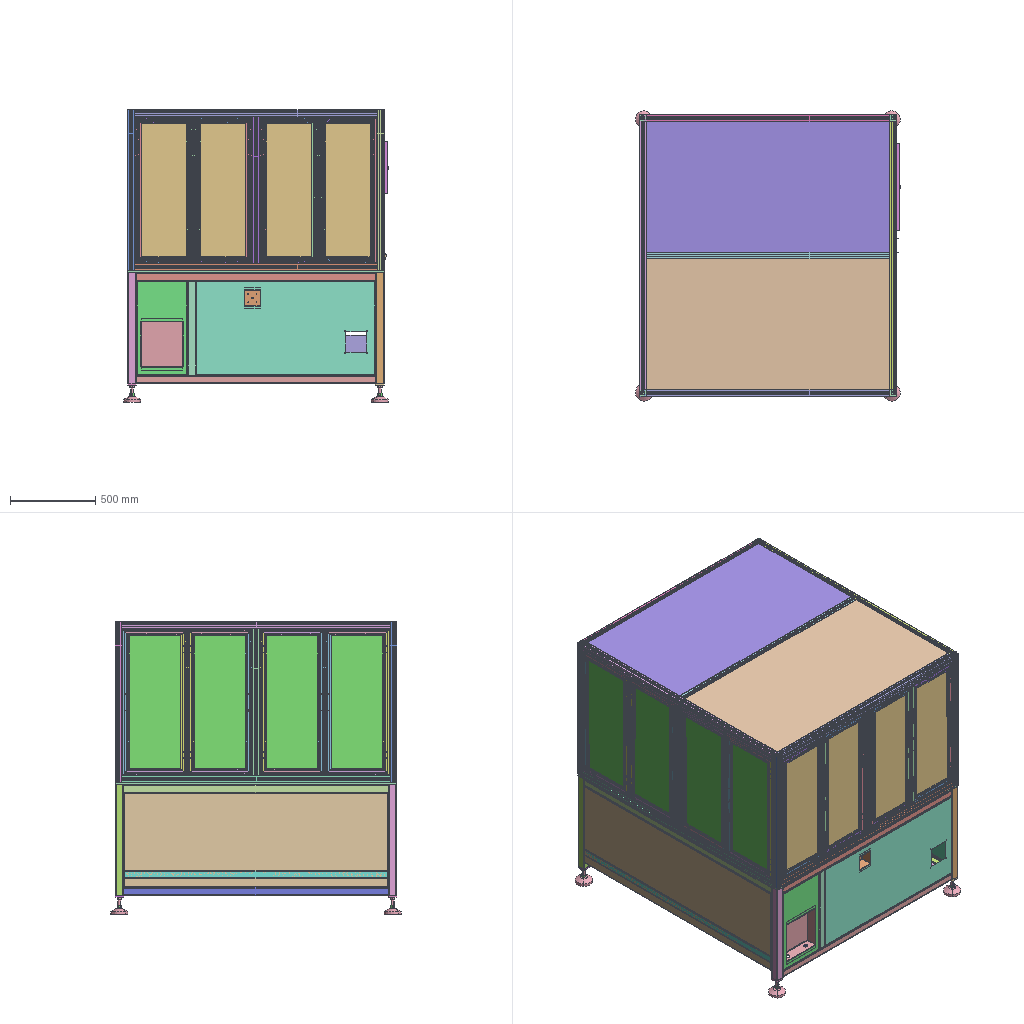Assembly | SolidWorks | 238 different items | 623 placed | box 1551 x 1700 x 1714 mm
Parts list (item | name | quantity | parent item | size | volume | features):
1 | (subassembly) | x2 | in 5 | 67.5 x 39 x 23.5 mm | 30109 mm3 | -
2 | (subassembly) | x1 | in 11 | 129 x 76.75 x 37 mm | 182069 mm3 | -
3 | (subassembly) | x2 | in 5, 21 | 99 x 76.75 x 37 mm | 182069 mm3 | -
4 | (subassembly) | x1 | in 21 | 152.5 x 57 x 74 mm | 389553 mm3 | -
5 | (subassembly) | x1 | - | 250 x 596.5 x 482 mm | 2400712 mm3 | -
6 | (subassembly) | x1 | in 15 | 103.415 x 32 x 20.8 mm | 30236 mm3 | -
7 | (subassembly) | x1 | in 15 | 10 x 102.865 x 20 mm | 11482 mm3 | -
8 | (subassembly) | x1 | in 36 | 226 x 45 x 54 mm | 65576 mm3 | -
9 | (subassembly) | x1 | in 37 | 181 x 45 x 54 mm | 67508 mm3 | -
10 | (subassembly) | x1 | in 37 | 83 x 83 x 36 mm | 177005 mm3 | -
11 | (subassembly) | x1 | - | - | 7253169 mm3 | -
12 | (subassembly) | x2 | in 35 | 83 x 83 x 36 mm | 177005 mm3 | features AEMSimFeature 1
13 | (subassembly) | x1 | - | - | 1570988 mm3 | features 3DProfileFeature 1
14 | (subassembly) | x1 | in 13 | 65 x 253 x 120 mm | 447705 mm3 | -
15 | (subassembly) | x1 | in 16 | 159.5 x 226.8 x 118.648 mm | 777455 mm3 | -
16 | (subassembly) | x1 | - | 159.5 x 226.8 x 118.648 mm | 777455 mm3 | -
17 | (subassembly) | x2 | in 18 | 102.5 x 118.189 x 195.029 mm | 527547 mm3 | -
18 | (subassembly) | x2 | - | 263 x 234.482 x 189.769 mm | 1000691 mm3 | -
19 | (subassembly) | x1 | - | - | - | features ReferencePattern 15, LocalCirPattern 2
20 | (subassembly) | x6 | in 19 | 80 x 60 x 32.8 mm | 73982 mm3 | features InContextFeatHolder 6
21 | (subassembly) | x1 | - | 353.5 x 596.5 x 482 mm | 3186701 mm3 | -
22 | (subassembly) | x1 | in 32 | 157 x 64 x 71 mm | 285801 mm3 | -
23 | (subassembly) | x1 | - | - | 100211807 mm3 | features ReferencePattern 10, MirrorCompFeat 4
24 | (subassembly) | x6 | in 19 | 40 x 111 x 58 mm | 78874 mm3 | features AEMSimFeature 1
25 | (subassembly) | x2 | - | 416.776 x 240 x 301.448 mm | 7009684 mm3 | -
26 | (subassembly) | x1 | - | 446.235 x 240 x 306.436 mm | 7009684 mm3 | -
27 | (subassembly) | x2 | in 5, 21 | 226 x 45 x 54 mm | 65576 mm3 | -
28 | (subassembly) | x1 | in 26 | 250 x 240 x 250 mm | 5886519 mm3 | -
29 | (subassembly) | x2 | in 25 | 250 x 240 x 250 mm | 5886519 mm3 | -
30 | (subassembly) | x6 | in 20 | 36 x 34.75 x 6.9 mm | 2892 mm3 | -
31 | (subassembly) | x1 | in 36 | 99 x 76.75 x 37 mm | 182069 mm3 | -
32 | (subassembly) | x1 | - | 285 x 559 x 312.685 mm | 2790889 mm3 | features ReferencePattern 5, CompositeCurve 2, MirrorCompFeat 1
33 | (subassembly) | x1 | in 36 | 152.5 x 57 x 74 mm | 389553 mm3 | -
34 | (subassembly) | x1 | - | 121 x 182 x 331.393 mm | 727155 mm3 | -
35 | (subassembly) | x2 | - | 121 x 83 x 36 mm | 201271 mm3 | -
36 | (subassembly) | x1 | - | 353.5 x 596.5 x 482 mm | 3186701 mm3 | features 3DProfileFeature 1
37 | (subassembly) | x1 | in 34 | 121 x 182 x 331.393 mm | 727155 mm3 | -
38 | - | x1 | in 22 | 157 x 50 x 50 mm | 85100 mm3 | features BaseBody 1
39 | - | x1 | - | 450 x 85 x 12 mm | 456645 mm3 | features BaseBody 1
40 | - | x1 | in 11 | 318 x 12 x 90 mm | 338579 mm3 | features HoleWzd 4, Chamfer 1, Extrusion 1
41 | - | x1 | - | 318 x 12 x 90 mm | 338579 mm3 | features BaseBody 1
42 | - | x1 | in 11 | 130 x 12 x 170 mm | 194409 mm3 | features HoleWzd 5, Chamfer 1, Extrusion 1
43 | - | x1 | - | 130 x 12 x 170 mm | 194409 mm3 | features BaseBody 1
44 | - | x1 | in 11 | 12 x 121.5 x 76 mm | 106329 mm3 | features HoleWzd 4, Chamfer 1, Extrusion 1
45 | - | x1 | - | 12 x 121.5 x 76 mm | 106329 mm3 | features BaseBody 1
46 | - | x1 | in 11 | 70 x 90 x 12 mm | 50116 mm3 | features HoleWzd 2, Chamfer 1, Extrusion 1
47 | - | x1 | - | 70 x 90 x 12 mm | 50116 mm3 | features BaseBody 1
48 | - | x1 | in 11 | 67 x 12 x 65 mm | 49086 mm3 | features HoleWzd 3, Extrusion 1
49 | - | x1 | in 22 | 80.5 x 71 x 64 mm | 175282 mm3 | features BaseBody 1
50 | - | x1 | - | 67 x 12 x 65 mm | 49086 mm3 | features BaseBody 1
51 | - | x2 | in 36 | 34 x 23.7 x 66.7 mm | 38485 mm3 | features BaseBody 2
52 | - | x2 | in 36 | 15 x 15 x 280 mm | 57550 mm3 | features BaseBody 1
53 | - | x1 | in 13 | - | - | features BaseBody 3, RefSurface 1
54 | - | x1 | in 13 | - | - | features BaseBody 14, RefSurface 4
55 | - | x1 | in 13 | 292.891 x 46.5 x 70 mm | 38586 mm3 | features BaseBody 7
56 | - | x1 | in 36 | 15 x 15 x 25 mm | 4329 mm3 | features BaseBody 1
57 | - | x4 | in 17 | 15 x 2.5 x 45 mm | 1095 mm3 | features BaseBody 1
58 | - | x2 | in 17 | 160 x 30 x 56 mm | 169757 mm3 | features BaseBody 1
59 | - | x4 | in 17 | 153.66 x 6 x 80 mm | 57575 mm3 | features BaseBody 1
60 | - | x2 | in 37 | 34 x 23.7 x 66.7 mm | 38485 mm3 | features BaseBody 2
61 | - | x12 | in 17 | 46 x 2 x 10 mm | 787.268 mm3 | features BaseBody 1
62 | - | x32 | in 17 | 46 x 0.5 x 10 mm | 196.817 mm3 | features BaseBody 1
63 | - | x2 | in 17 | 80 x 15 x 180 mm | 182488 mm3 | features BaseBody 1
64 | - | x4 | in 17 | 46 x 2 x 70 mm | 6168 mm3 | features BaseBody 1
65 | - | x4 | in 17 | 46 x 1.5 x 102 mm | 6734 mm3 | features BaseBody 1
66 | - | x2 | in 37 | 15 x 15 x 280 mm | 57550 mm3 | features BaseBody 1
67 | - | x2 | in 18 | 116 x 15 x 60 mm | 18438 mm3 | features BaseBody 1
68 | - | x2 | in 18 | 189.769 x 2 x 46.25 mm | 14558 mm3 | features BaseBody 1
69 | - | x2 | in 18 | 263 x 106.293 x 188.106 mm | 187834 mm3 | features BaseBody 1
70 | - | x2 | in 32 | 12 x 12 x 40 mm | 4457 mm3 | features Extrusion 1, RevCut 1
71 | - | x1 | in 36 | 28 x 30 x 10 mm | 7787 mm3 | features BaseBody 1
72 | - | x1 | in 19 | 700 x 690 x 12 mm | 4521944 mm3 | features CirPattern 5, ICE 3, HoleWzd 2, Extrusion 1
73 | - | x1 | in 23 | 1500 x 1650 x 672 mm | 49489000 mm3 | features ICE 14, FlatPattern 12, EdgeFlange 11, HoleWzd 11, SMBaseFlange 9, SheetMetal 9, MirrorSolid 6, MirrorPattern 4, Fillet 3, MoveCopyBody 2, MoveFace 2, WeldCornerFeat 2, 3DProfileFeature 1, Chamfer 1, EndCap 1, WeldMemberFeat 1, WeldmentFeature 1
74 | - | x6 | in 20 | 60 x 50 x 32 mm | 31490 mm3 | features Cut 4, ICE 4, Extrusion 1, Fillet 1, MirrorPattern 1
75 | - | x6 | in 20 | 80 x 60 x 20 mm | 39600 mm3 | features ICE 2, Extrusion 1
76 | - | x2 | - | 250 x 134 x 174.039 mm | 134233 mm3 | features BaseBody 3
77 | - | x1 | in 23 | 1500 x 1650 x 942 mm | 12502911 mm3 | features WeldCornerFeat 2, 3DProfileFeature 1, ICE 1, MirrorSolid 1, WeldMemberFeat 1, WeldmentFeature 1
78 | - | x5 | in 23 | 379.5 x 856 x 20 mm | 2107206 mm3 | features HoleWzd 3, ICE 1, WeldMemberFeat 1, WeldmentFeature 1
79 | - | x2 | in 35 | 80 x 30 x 10 mm | 23980 mm3 | features Extrusion 1, ICE 1
80 | - | x4 | in 35 | 2.5 x 2.5 x 30 mm | 142.655 mm3 | features Chamfer 1, Extrusion 1
81 | - | x1 | in 23 | 379.5 x 856 x 20 mm | 2241124 mm3 | features HoleWzd 3, ICE 3, WeldMemberFeat 1, WeldmentFeature 1
82 | - | x1 | - | 20 x 20 x 65 mm | 20420 mm3 | features BaseBody 1
83 | - | x8 | in 23 | 341.5 x 856 x 20 mm | 1950280 mm3 | features HoleWzd 3, ICE 1, WeldMemberFeat 1, WeldmentFeature 1
84 | - | x1 | in 23 | 764 x 860 x 5 mm | 2935200 mm3 | features Extrusion 1, ICE 1
85 | - | x2 | in 23 | 384.5 x 547 x 21.5 mm | 378210 mm3 | features EdgeFlange 3, ICE 2, Fillet 1, FlatPattern 1, SMBaseFlange 1, SheetMetal 1
86 | - | x2 | in 23 | 371 x 547 x 20 mm | 376908 mm3 | features EdgeFlange 2, ICE 2, FlatPattern 1, SMBaseFlange 1, SheetMetal 1
87 | - | x1 | in 37 | 180 x 30 x 20 mm | 107950 mm3 | features Extrusion 1, ICE 1
88 | - | x2 | in 37 | 4 x 4 x 20 mm | 251.327 mm3 | features Extrusion 1
89 | - | x6 | in 19 | 25 x 40 x 18 mm | 6202 mm3 | features ICE 2, Chamfer 1, Extrusion 1
90 | - | x6 | in 5, 21, 36 | 60 x 34 x 15 mm | 30600 mm3 | features Extrusion 1
91 | - | x1 | in 21 | 28 x 30 x 10 mm | 7787 mm3 | features BaseBody 1
92 | - | x1 | in 37 | 180 x 100 x 10 mm | 124316 mm3 | features Extrusion 1, HoleWzd 1, ICE 1
93 | - | x4 | in 12 | 40.5 x 5.8 x 4.4 mm | 628.814 mm3 | features BaseBody 1
94 | - | x1 | in 37 | 23 x 30 x 10 mm | 6287 mm3 | features Chamfer 1, Extrusion 1, HoleWzd 1
95 | - | x2 | in 37 | 20 x 20 x 65 mm | 20420 mm3 | features Extrusion 1
96 | - | x6 | in 24 | 40 x 65 x 40 mm | 52409 mm3 | features BaseBody 1
97 | - | x6 | in 24 | 50.3 x 73.5 x 24.6 mm | 26465 mm3 | features BaseBody 1
98 | - | x2 | in 10 | 40.5 x 5.8 x 4.4 mm | 628.814 mm3 | features BaseBody 1
99 | - | x1 | in 2 | 98 x 76.35 x 36.35 mm | 83829 mm3 | features BaseBody 1
100 | - | x2 | in 3 | 98 x 76.35 x 36.35 mm | 83829 mm3 | features BaseBody 1
101 | - | x1 | in 2 | 93.95 x 76.75 x 36.25 mm | 97741 mm3 | features BaseBody 1
102 | - | x2 | in 3 | 93.95 x 76.75 x 36.25 mm | 97741 mm3 | features BaseBody 1
103 | - | x1 | in 4 | 152.5 x 57 x 74 mm | 389553 mm3 | features BaseBody 1
104 | - | x2 | in 21 | 7 x 8.083 x 8 mm | 182.321 mm3 | features BaseBody 1
105 | - | x1 | in 2 | 4 x 5.4 x 50 mm | 499.04 mm3 | features BaseBody 1
106 | - | x2 | in 3 | 4 x 5.4 x 50 mm | 499.04 mm3 | features BaseBody 1
107 | - | x2 | in 27 | 25 x 45 x 54 mm | 7496 mm3 | features BaseBody 1
108 | - | x1 | in 23 | 508 x 304 x 60 mm | 4453867 mm3 | features ICE 10, BaseBody 1, HoleWzd 1
109 | - | x45 | in 25, 26 | 0.76 x 0.76 x 10.15 mm | 4.895 mm3 | features BaseBody 1
110 | - | x1 | in 28 | 250 x 240 x 250 mm | 5886519 mm3 | features BaseBody 7
111 | - | x2 | in 29 | 250 x 240 x 250 mm | 5886519 mm3 | features BaseBody 7
112 | - | x24 | in 25, 26 | 10.001 x 11.547 x 5.7 mm | 368.052 mm3 | features BaseBody 1
113 | - | x3 | in 25, 26 | 95 x 118.301 x 180 mm | 694556 mm3 | features BaseBody 64
114 | - | x1 | in 19 | - | - | features MBimport 1
115 | - | x2 | in 21 | 10 x 10 x 46 mm | 1521 mm3 | features BaseBody 1
116 | - | x1 | in 21 | 24 x 24 x 51 mm | 10675 mm3 | features BaseBody 1
117 | - | x4 | in 23 | 100 x 153 x 100 mm | 235299 mm3 | features ICE 3, Revolution 1
118 | - | x44 | in 17 | 9 x 20.5 x 9 mm | 774.01 mm3 | features BaseBody 1
119 | - | x2 | in 27 | 202 x 25 x 25 mm | 39660 mm3 | features BaseBody 1
120 | - | x4 | in 27 | 7 x 33.486 x 29 mm | 2689 mm3 | features BaseBody 1
121 | - | x2 | in 27 | 6 x 13.856 x 12 mm | 526.058 mm3 | features BaseBody 1
122 | - | x2 | in 27 | 191.2 x 19.5 x 19.5 mm | 12515 mm3 | features BaseBody 1
123 | - | x1 | in 10 | 67 x 36 x 83 mm | 131931 mm3 | features BaseBody 1
124 | - | x1 | in 10 | 81 x 30 x 81 mm | 43817 mm3 | features BaseBody 1
125 | - | x6 | in 30 | 36 x 16.5 x 3.5 mm | 1384 mm3 | features BaseBody 1
126 | - | x4 | in 11 | 75 x 65 x 65 mm | 177791 mm3 | features BaseBody 1
127 | - | x6 | in 30 | 36 x 30.45 x 3 mm | 1415 mm3 | features BaseBody 1
128 | - | x3 | in 25, 26 | 110 x 15 x 155 mm | 241962 mm3 | features BaseBody 1
129 | - | x12 | in 25, 26 | 12 x 66 x 12 mm | 5184 mm3 | features BaseBody 1
130 | - | x3 | in 25, 26 | 110 x 10 x 155 mm | 162886 mm3 | features BaseBody 1
131 | - | x1 | in 15 | 133 x 16 x 16 mm | 13170 mm3 | features ICE 2, Chamfer 1, Revolution 1
132 | - | x1 | in 15 | 150 x 12 x 80 mm | 130957 mm3 | features HoleWzd 3, Chamfer 1, Extrusion 1, ICE 1
133 | - | x1 | - | 15 x 202 x 80 mm | 199416 mm3 | features HoleWzd 4, ICE 3, Chamfer 1, Cut 1, Extrusion 1
134 | - | x1 | in 15 | 67 x 10 x 80 mm | 51889 mm3 | features HoleWzd 2, Extrusion 1, MirrorPattern 1
135 | - | x1 | in 15 | 60 x 53 x 53 mm | 64620 mm3 | features ICE 5, Chamfer 2, Extrusion 1, HoleWzd 1
136 | - | x1 | in 15 | 11 x 80 x 23 mm | 16527 mm3 | features HoleWzd 3, Chamfer 1, Extrusion 1, ICE 1
137 | - | x5 | in 5, 21 | 75 x 65 x 65 mm | 177791 mm3 | features BaseBody 1
138 | - | x2 | in 15 | 15 x 202 x 80 mm | 195162 mm3 | features ICE 6, HoleWzd 4, Chamfer 2, Fillet 2, Cut 1, Extrusion 1
139 | - | x2 | in 15 | 97 x 10 x 20 mm | 17099 mm3 | features HoleWzd 2, Chamfer 1, Extrusion 1, ICE 1
140 | - | x1 | in 15 | 15 x 25 x 6 mm | 1891 mm3 | features HoleWzd 2, Chamfer 1, Extrusion 1, ICE 1
141 | - | x1 | in 15 | 20 x 67 x 8 mm | 10486 mm3 | features HoleWzd 2, Chamfer 1, Extrusion 1
142 | - | x1 | in 15 | 9.238 x 8 x 4.7 mm | 190.671 mm3 | features BaseBody 1
143 | - | x4 | in 5, 21 | 34 x 23.7 x 66.7 mm | 38485 mm3 | features BaseBody 2
144 | - | x4 | in 5, 21 | 15 x 15 x 280 mm | 57550 mm3 | features BaseBody 1
145 | - | x2 | in 18 | 140 x 10 x 185 mm | 252313 mm3 | features BaseBody 1
146 | - | x12 | in 30 | 4 x 6.9 x 4 mm | 46.627 mm3 | features BaseBody 1
147 | - | x2 | in 11, 21 | 15 x 15 x 25 mm | 4329 mm3 | features BaseBody 1
148 | - | x2 | in 36 | 10 x 10 x 46 mm | 1521 mm3 | features BaseBody 1
149 | - | x2 | in 11 | 35 x 275 x 35 mm | 118575 mm3 | features Extrusion 1, Shell 1
150 | - | x1 | - | 15 x 15 x 25 mm | 4329 mm3 | features Extrusion 1, HoleWzd 1
151 | - | x2 | in 17 | 18.5 x 27 x 18.5 mm | 7258 mm3 | features BaseBody 1
152 | - | x1 | - | 35 x 275 x 35 mm | 118575 mm3 | features BaseBody 1
153 | - | x6 | in 5, 21, 36 | 35 x 515 x 35 mm | 222060 mm3 | features Extrusion 1, Shell 1
154 | - | x1 | - | 35 x 515 x 35 mm | 222060 mm3 | features BaseBody 1
155 | - | x4 | in 5, 21 | 85 x 75 x 50 mm | 169404 mm3 | features BaseBody 1
156 | - | x4 | in 5, 21 | 53.5 x 57 x 57.999 mm | 57966 mm3 | features BaseBody 1
157 | - | x2 | in 1 | 50 x 39 x 23.5 mm | 27612 mm3 | features BaseBody 1
158 | - | x2 | in 1 | 21 x 15.4 x 10.1 mm | 1248 mm3 | features BaseBody 1
159 | - | x2 | in 1 | 21 x 15.4 x 10.1 mm | 1248 mm3 | features BaseBody 1
160 | - | x1 | in 31 | 98 x 76.35 x 36.35 mm | 83829 mm3 | features BaseBody 1
161 | - | x3 | in 36 | 75 x 65 x 65 mm | 177791 mm3 | features BaseBody 1
162 | - | x1 | in 31 | 93.95 x 76.75 x 36.25 mm | 97741 mm3 | features BaseBody 1
163 | - | x1 | in 33 | 152.5 x 57 x 74 mm | 389553 mm3 | features BaseBody 1
164 | - | x1 | in 31 | 4 x 5.4 x 50 mm | 499.04 mm3 | features BaseBody 1
165 | - | x1 | in 15 | 2.8 x 10.8 x 2.8 mm | 49.198 mm3 | features BaseBody 1
166 | - | x1 | in 6 | 65 x 32 x 20 mm | 25563 mm3 | features BaseBody 1
167 | - | x2 | in 15 | 6 x 22 x 22 mm | 1447 mm3 | features BaseBody 1
168 | - | x1 | in 15 | 34.5 x 14.8 x 14 mm | 3294 mm3 | features BaseBody 1
169 | - | x1 | in 15 | 18 x 18 x 10 mm | 1499 mm3 | features BaseBody 1
170 | - | x2 | in 7 | 20 x 8 x 28.9 mm | 3299 mm3 | features BaseBody 1
171 | - | x1 | in 7 | 9 x 6.5 x 100 mm | 4884 mm3 | features BaseBody 1
172 | - | x2 | in 36 | 85 x 75 x 50 mm | 169404 mm3 | features BaseBody 1
173 | - | x1 | in 15 | 26.982 x 26.934 x 20 mm | 6760 mm3 | features BaseBody 1
174 | - | x1 | in 15 | 60 x 12 x 10 mm | 6024 mm3 | features BaseBody 1
175 | - | x2 | in 6 | 40.5 x 5.8 x 4.4 mm | 628.814 mm3 | features BaseBody 1
176 | - | x1 | in 6 | 4 x 9.238 x 8 mm | 163.484 mm3 | features BaseBody 1
177 | - | x1 | in 6 | 72 x 15.6 x 15.6 mm | 3252 mm3 | features BaseBody 1
178 | - | x2 | in 15 | 62.75 x 5.5 x 40.5 mm | 476.928 mm3 | features BaseBody 2
179 | - | x2 | in 36 | 62.75 x 5.5 x 40.5 mm | 476.928 mm3 | features BaseBody 2
180 | - | x2 | in 11 | - | 325247 mm3 | features BaseBody 3
181 | - | x3 | in 8, 9 | 25 x 45 x 54 mm | 7496 mm3 | features BaseBody 1
182 | - | x1 | in 13 | 75 x 65 x 65 mm | 177791 mm3 | features BaseBody 1
183 | - | x2 | in 36 | 53.5 x 57 x 57.999 mm | 57966 mm3 | features BaseBody 1
184 | - | x1 | in 13 | 35 x 337 x 35 mm | 145309 mm3 | features Extrusion 1, Shell 1
185 | - | x2 | in 13 | 85 x 75 x 50 mm | 169404 mm3 | features BaseBody 1
186 | - | x1 | in 11 | 364.5 x 78 x 161.5 mm | 1915592 mm3 | features BaseBody 14
187 | - | x1 | in 11 | 464.5 x 78 x 161.5 mm | 2357243 mm3 | features BaseBody 14
188 | - | x1 | in 36 | 24 x 24 x 51 mm | 10675 mm3 | features BaseBody 1
189 | - | x1 | in 37 | 24 x 24 x 51 mm | 10675 mm3 | features BaseBody 1
190 | - | x1 | in 8 | 202 x 25 x 25 mm | 39660 mm3 | features BaseBody 1
191 | - | x1 | in 9 | 152 x 25 x 25 mm | 36609 mm3 | features BaseBody 1
192 | - | x2 | in 8 | 7 x 33.486 x 29 mm | 2689 mm3 | features BaseBody 1
193 | - | x2 | in 9 | 7 x 33.486 x 29 mm | 2689 mm3 | features BaseBody 1
194 | - | x1 | in 32 | 34 x 23.7 x 61.7 mm | 37046 mm3 | features BaseBody 1
195 | - | x1 | in 8 | 6 x 13.856 x 12 mm | 526.058 mm3 | features BaseBody 1
196 | - | x1 | in 9 | 6 x 13.856 x 12 mm | 526.058 mm3 | features BaseBody 1
197 | - | x1 | in 8 | 191.2 x 19.5 x 19.5 mm | 12515 mm3 | features BaseBody 1
198 | - | x1 | in 9 | 141.2 x 19.5 x 19.5 mm | 10002 mm3 | features BaseBody 1
199 | - | x2 | in 12 | 67 x 36 x 83 mm | 131931 mm3 | features BaseBody 1
200 | - | x2 | in 12 | 81 x 30 x 81 mm | 43817 mm3 | features BaseBody 1
201 | - | x1 | in 13 | 125 x 100 x 120 mm | 52954 mm3 | features ICE 3, HoleWzd 2, Chamfer 1, EdgeFlange 1, Fillet 1, FlatPattern 1, MirrorSolid 1, SMBaseFlange 1, SheetMetal 1
202 | - | x1 | in 32 | 18 x 70 x 150 mm | 155887 mm3 | features HoleWzd 3, Chamfer 1, Cut 1, Extrusion 1, ICE 1
203 | - | x2 | in 32 | 32 x 50 x 10 mm | 10890 mm3 | features HoleWzd 2, Chamfer 1, Extrusion 1
204 | - | x1 | in 32 | 12 x 150 x 156 mm | 257350 mm3 | features HoleWzd 2, Chamfer 1, Extrusion 1, ICE 1
205 | - | x2 | in 32 | 15 x 15 x 130 mm | 23633 mm3 | features BaseBody 1
206 | - | x2 | in 32 | 60 x 380 x 35 mm | 206976 mm3 | features HoleWzd 2, ICE 2, Chamfer 1, Extrusion 1
207 | - | x2 | in 32 | 95 x 380 x 60 mm | 225421 mm3 | features HoleWzd 3, ICE 3, Chamfer 1, Extrusion 1
208 | - | x1 | in 32 | 25 x 150 x 20 mm | 66993 mm3 | features HoleWzd 3, Chamfer 1, Extrusion 1, Fillet 1, ICE 1
209 | - | x1 | in 13 | 85 x 230 x 12 mm | 215246 mm3 | features HoleWzd 3, Chamfer 1, Extrusion 1, ICE 1
210 | - | x1 | in 13 | 50 x 42 x 52.5 mm | 37086 mm3 | features HoleWzd 2, ICE 2, Chamfer 1, Extrusion 1
211 | - | x1 | in 32 | 250 x 15 x 280 mm | 665009 mm3 | features HoleWzd 6, ICE 4, Chamfer 2, Extrusion 1
212 | - | x1 | in 32 | 230 x 15 x 100 mm | 269787 mm3 | features HoleWzd 7, ICE 2, Chamfer 1, Extrusion 1
213 | - | x1 | in 32 | 50 x 12 x 120 mm | 62317 mm3 | features HoleWzd 5, Chamfer 1, Extrusion 1
214 | - | x1 | in 14 | 65 x 12 x 120 mm | 87146 mm3 | features HoleWzd 2, Chamfer 1, Cut 1, Extrusion 1
215 | - | x2 | in 14 | 65 x 233 x 10 mm | 150775 mm3 | features HoleWzd 2, Extrusion 1, MirrorPattern 1
216 | - | x1 | in 22 | 8 x 31.177 x 27 mm | 3647 mm3 | features BaseBody 1
217 | - | x1 | in 14 | 95 x 10 x 65 mm | 59009 mm3 | features HoleWzd 2, Chamfer 1, Extrusion 1
218 | - | x1 | - | 95 x 10 x 65 mm | 59009 mm3 | features BaseBody 1
219 | - | x1 | in 32 | 34.641 x 80 x 30 mm | 47834 mm3 | features ICE 1, Revolution 1
220 | - | x6 | in 5, 21, 36 | 92.5 x 40 x 65 mm | 11298 mm3 | features ICE 2, Fillet 1, FlatPattern 1, HoleWzd 1, SMBaseFlange 1, SheetMetal 1
221 | - | x1 | - | 92.5 x 40 x 65 mm | 11298 mm3 | features BaseBody 1
222 | - | x3 | in 5, 21, 36 | 300 x 115 x 12 mm | 411276 mm3 | features HoleWzd 3, Chamfer 1, Extrusion 1
223 | - | x2 | in 21, 36 | 68.5 x 29 x 15 mm | 15619 mm3 | features HoleWzd 2, Chamfer 1, Extrusion 1, ICE 1
224 | - | x2 | in 21, 36 | 78 x 29 x 20 mm | 18504 mm3 | features ICE 3, HoleWzd 2, Chamfer 1, Extrusion 1, Fillet 1
225 | - | x3 | in 5, 21, 36 | 65 x 12 x 68.5 mm | 35580 mm3 | features HoleWzd 3, ICE 2, Chamfer 1, Extrusion 1
226 | - | x1 | - | 65 x 12 x 68.5 mm | 35580 mm3 | features BaseBody 1
227 | - | x1 | in 22 | 31 x 36 x 36 mm | 21780 mm3 | features BaseBody 1
228 | - | x3 | in 5, 21, 36 | 10 x 145 x 76 mm | 109672 mm3 | features HoleWzd 2, Chamfer 1, Extrusion 1
229 | - | x1 | - | 10 x 145 x 76 mm | 109672 mm3 | features BaseBody 1
230 | - | x1 | - | 130 x 12 x 70 mm | 95885 mm3 | features BaseBody 1
231 | - | x2 | in 21, 36 | 130 x 12 x 70 mm | 95885 mm3 | features HoleWzd 3, Chamfer 1, Cut 1, Extrusion 1, ICE 1
232 | - | x2 | in 21, 36 | 12 x 80 x 70 mm | 63301 mm3 | features HoleWzd 3, Chamfer 1, Extrusion 1
233 | - | x2 | in 21, 36 | 65 x 15 x 82.5 mm | 36373 mm3 | features HoleWzd 4, Cut 2, Chamfer 1, Extrusion 1
234 | - | x4 | in 21, 36 | 70 x 40 x 8 mm | 14827 mm3 | features HoleWzd 2, Chamfer 1, Extrusion 1
235 | - | x4 | in 5 | 12 x 27 x 10.5 mm | 1656 mm3 | features ICE 3, Chamfer 1, Extrusion 1, HoleWzd 1
236 | - | x1 | - | 12 x 27 x 10.5 mm | 1648 mm3 | features BaseBody 1
237 | - | x1 | in 11 | 450 x 85 x 12 mm | 456645 mm3 | features HoleWzd 3, Chamfer 1, Extrusion 1
238 | - | x2 | in 36 | 7 x 8.083 x 8 mm | 182.321 mm3 | features BaseBody 1
Mates (type | each side: item.copy, entity, surface, feature):
In the top assembly
Concentric | 73.1 face cylinder Cut-Extrude 14 | 72.1 face cylinder Boss-Extrude 1
Coincident | 73.1 face plane Boss-Extrude 2 | 114.1 face plane JE - 70DF 水平带轮式Right侧后方WS (FlangeFace及壳体加定位销).STEP<1>
Parallel | 73.1 face plane 冷弯空心方管gb∕t6728-2002 50 X 50 X 3(1) | 72.1 face plane CirPattern 1
Coincident | 73.1 face plane Boss-Extrude 2 | 199.1 face plane TC-L-20x3030_b
Width | 199.1 face plane TC-L-20x3030_b | 199.1 face plane TC-L-20x3030_b | 75.1 face plane Boss-Extrude 1 | 75.1 face plane Boss-Extrude 1
Width | 75.1 face plane Boss-Extrude 1 | 75.1 face plane Boss-Extrude 1 | assembly face | assembly face
Coincident | 73.1 face plane Boss-Extrude 2 | 128.1 face plane 输入1
Width | 128.1 face plane 输入1 | 128.1 face plane 输入1 | 75.1 face plane Boss-Extrude 1 | 75.1 face plane Boss-Extrude 1
DistanceDim | 113.1 face plane 输入64 | 75.1 face plane Boss-Extrude 1
Coincident | 73.1 face plane Boss-Extrude 2 | 128.2 face plane 输入1
DistanceDim | 113.2 face plane 输入64 | 75.2 face plane Boss-Extrude 1
Coincident | 73.1 face plane Boss-Extrude 2 | 128.3 face plane 输入1
Coincident | 73.1 face plane Boss-Extrude 2 | 137.1 face plane 输入1
Parallel | 113.3 face plane 输入14 | 222.1 face
Coincident | 73.1 face plane Boss-Extrude 2 | assembly edge
Width | 202.1 face | 202.1 face | 75.3 face plane Boss-Extrude 1 | 75.3 face plane Boss-Extrude 1
Coincident | 73.1 face plane Boss-Extrude 2 | 214.1 face
Width | 215.1 face | 215.2 face | 75.4 face plane Boss-Extrude 1 | 75.4 face plane Boss-Extrude 1
Coincident | 73.1 face plane Boss-Extrude 2 | 126.1 face plane 输入1
Parallel | 75.5 face plane Boss-Extrude 1 | 237.1 face
DistanceDim | 126.1 face plane 输入1 | 73.1 face plane 冷弯空心方管gb∕t6728-2002 50 X 50 X 3(1)
Coincident | 73.1 face plane Boss-Extrude 2 | 76.1 face plane 输入3
Coincident | 73.1 face plane 冷弯空心方管gb∕t6728-2002 50 X 50 X 3(1) | 76.1 edge
Coincident | 73.1 face plane Boss-Extrude 2 | 76.2 face plane 输入2
Coincident | 76.1 face plane 输入2 | 76.2 face plane 输入3
DistanceDim | 76.2 face plane 输入3 | 76.1 face plane 输入2
DistanceDim | 76.2 face plane 输入2 | 126.1 face plane 输入1
Coincident | 73.1 face plane Boss-Extrude 2 | 145.1 face plane 输入1
Parallel | 73.1 face plane Boss-Extrude 2 | 145.1 face plane 输入1
DistanceDim | 145.1 face plane 输入1 | 73.1 face plane Boss-Extrude 2
Coincident | 73.1 face plane Boss-Extrude 2 | 145.2 face plane 输入1
Coincident | 145.1 face plane 输入1 | 145.2 face plane 输入1
Coincident | 73.1 face plane Boss-Extrude 2 | 132.1 face
Width | 138.1 face | 138.2 face | 75.6 face plane Boss-Extrude 1 | 75.6 face plane Boss-Extrude 1
DistanceDim | 128.3 face plane 输入1 | 132.1 face
Width | 138.1 face | 138.2 face | 130.1 face plane 输入1 | 113.3 face plane 输入63
Coincident | 73.1 face plane Boss-Extrude 2 | 66.1 face plane 输入1
Width | 87.1 face | 87.1 face | 75.3 face plane Boss-Extrude 1 | 75.3 face plane Boss-Extrude 1
Coincident | 73.1 face plane Boss-Extrude 2 | 206.1 face plane Boss-Extrude 2
Width | 211.1 face plane Boss-Extrude 1 | 211.1 face plane Boss-Extrude 1 | 75.3 face plane Boss-Extrude 1 | 75.3 face plane Boss-Extrude 1
Coincident | 73.1 face plane Boss-Extrude 2 | 161.1 face plane 输入1
Parallel | 128.1 face plane 输入1 | 161.2 face plane 输入1
Coincident | 73.1 face plane Boss-Extrude 2 | 137.2 face plane 输入1
Parallel | 128.2 face plane 输入1 | 137.2 face plane 输入1
In subassembly 35
Coincident | 200.1 face plane TCL-20x30-0_30fp | 79.1 face plane Boss-Extrude 1
Width | 200.1 face plane TCL-20x30-0_30fp | 200.1 face plane TCL-20x30-0_30fp | 79.1 face plane Boss-Extrude 1 | 79.1 face plane Boss-Extrude 1 | 2 times
Concentric | 79.1 face cylinder Cut-Extrude 1 | 80.1 face cylinder Boss-Extrude 1
Coincident | 79.1 face plane Cut-Extrude 1 | 80.1 face plane Boss-Extrude 1
Concentric | 79.1 face cylinder Cut-Extrude 1 | 80.2 face cylinder Boss-Extrude 1
Coincident | 79.1 face plane Cut-Extrude 1 | 80.2 face plane Boss-Extrude 1
In subassembly 23
Concentric | 73.2 face cylinder Mirror 1 | 117.1 face cylinder Boss-Extrude 2
Coincident | 73.2 face plane Mirror 1 | 117.1 face plane Boss-Extrude 3
Concentric | 73.2 face cylinder Mirror 3 | 117.2 face cylinder Boss-Extrude 2
Coincident | 117.1 face plane Revolve 1 | 117.2 face plane Revolve 1
Concentric | 73.2 face cylinder Mirror 2 | 117.3 face cylinder Boss-Extrude 2
Coincident | 117.1 face plane Revolve 1 | 117.3 face plane Revolve 1
Concentric | 73.2 face cylinder Mirror 3 | 117.4 face cylinder Boss-Extrude 2
Coincident | 117.3 face plane Revolve 1 | 117.4 face plane Revolve 1
Coincident | 73.2 face plane Boss-Extrude 2 | 77.1 face plane 工业Aluminium Profile 40 X 40A X R0.5(1)
Coincident | 73.2 face plane 冷弯空心方管gb∕t6728-2002 50 X 50 X 3(1) | 77.1 face plane 工业Aluminium Profile 40 X 40A X R0.5(1) | 2 times
Width | 78.1 face plane Aluminium Profile 2040A(1) | 78.1 face plane Aluminium Profile 2040A(1) | 77.1 face plane 工业Aluminium Profile 40 X 40A X R0.5(1) | 77.1 face plane 工业Aluminium Profile 40 X 40A X R0.5(1)
Coincident | 77.1 face plane 工业Aluminium Profile 40 X 40A X R0.5(1) | 78.1 face plane Aluminium Profile 2040A(1)
DistanceDim | 78.1 face plane Aluminium Profile 2040A(1) | 77.1 face plane 工业Aluminium Profile 40 X 40A X R0.5(1)
Coincident | 78.1 face plane Aluminium Profile 2040A(1) | 81.1 face plane Aluminium Profile 2040A(1) | 2 times
DistanceDim | 81.1 face plane Aluminium Profile 2040A(1) | 77.1 face plane 工业Aluminium Profile 40 X 40A X R0.5(1)
Coincident | 77.1 face plane 工业Aluminium Profile 40 X 40A X R0.5(1) | 83.1 face plane Aluminium Profile 2040A(1)
DistanceDim | 83.1 face plane Aluminium Profile 2040A(1) | 77.1 face plane 工业Aluminium Profile 40 X 40A X R0.5(1)
Coincident | 78.1 face plane Aluminium Profile 2040A(1) | 83.1 face plane Aluminium Profile 2040A(1)
Coincident | 83.1 face plane Aluminium Profile 2040A(1) | 83.2 face plane Aluminium Profile 2040A(1) | 2 times
DistanceDim | 83.2 face plane Aluminium Profile 2040A(1) | 77.1 face plane 工业Aluminium Profile 40 X 40A X R0.5(1)
Coincident | 77.1 face plane 工业Aluminium Profile 40 X 40A X R0.5(1) | 78.2 face plane Aluminium Profile 2040A(1)
Coincident | 83.3 face plane Aluminium Profile 2040A(1) | 78.2 face plane Aluminium Profile 2040A(1)
DistanceDim | 78.2 face plane Aluminium Profile 2040A(1) | 77.1 face plane 工业Aluminium Profile 40 X 40A X R0.5(1)
Coincident | 78.2 face plane Aluminium Profile 2040A(1) | 78.3 face plane Aluminium Profile 2040A(1) | 2 times
DistanceDim | 78.3 face plane Aluminium Profile 2040A(1) | 77.1 face plane 工业Aluminium Profile 40 X 40A X R0.5(1)
Coincident | 77.1 face plane 工业Aluminium Profile 40 X 40A X R0.5(1) | 84.1 face plane Boss-Extrude 1 | 3 times
Coincident | 84.1 face plane Boss-Extrude 1 | 108.1 face plane Boss-Extrude 1
Width | 77.1 face plane 工业Aluminium Profile 40 X 40A X R0.5(1) | 77.1 face plane 工业Aluminium Profile 40 X 40A X R0.5(1) | 108.1 face plane Boss-Extrude 1 | 108.1 face plane Boss-Extrude 1
Coincident | 73.2 face plane 冷弯空心方管gb∕t6728-2002 50 X 50 X 3(1) | 85.1 face plane Base-Flange 1
DistanceDim | 85.1 face plane Edge-Flange 1 | 73.2 face plane 冷弯空心方管gb∕t6728-2002 50 X 50 X 3(1)
Width | 73.2 face plane 冷弯空心方管gb∕t6728-2002 50 X 50 X 3(1) | 73.2 face plane 冷弯空心方管gb∕t6728-2002 50 X 50 X 3(1) | 85.1 face plane Edge-Flange 1 | 85.1 face plane Edge-Flange 1
Coincident | 85.1 face plane Base-Flange 1 | 86.1 face plane Base-Flange 1
Coincident | 85.1 face plane Edge-Flange 1 | 86.1 face plane Edge-Flange 1
In subassembly 19
Concentric | 114.2 face cylinder JE - 70DF 水平带轮式Right侧后方WS (FlangeFace及壳体加定位销).STEP<1> | 72.2 face cylinder Boss-Extrude 1
Coincident | 114.2 face plane JE - 70DF 水平带轮式Right侧后方WS (FlangeFace及壳体加定位销).STEP<1> | 72.2 face plane Boss-Extrude 1
Parallel | 114.2 face plane JE - 70DF 水平带轮式Right侧后方WS (FlangeFace及壳体加定位销).STEP<1> | 72.2 face plane CirPattern 1
Coincident | 72.2 face plane Boss-Extrude 1 | 75.7 face plane Boss-Extrude 1
Width | 75.7 face plane Boss-Extrude 1 | 75.7 face plane Boss-Extrude 1 | 72.2 face plane CirPattern 2 | 72.2 face plane CirPattern 2 | 2 times
Coincident | 72.2 face plane Boss-Extrude 1 | 96.1 face plane ACKx25_b
Width | 75.8 face plane Boss-Extrude 1 | 75.8 face plane Boss-Extrude 1 | 96.1 face plane ACKx25_b | 96.1 face plane ACKx25_b
Coincident | 75.8 face plane Boss-Extrude 1 | 96.1 face plane ACKx25_b
Concentric | 97.1 face cylinder ACKx25_r | 89.1 face cylinder Cut-Extrude 1
Coincident | 97.1 face plane ACKx25_r | 89.1 face plane Boss-Extrude 1
Parallel | 97.1 face plane ACKx25_r | 89.1 face plane Boss-Extrude 1
In subassembly 20
Concentric | 74.1 face | 127.1 face cylinder 输入1
Coincident | 74.1 face plane Cut-Extrude 1 | 127.1 face plane 输入1
Parallel | 74.1 face plane Boss-Extrude 1 | 125.1 face plane 输入1
Width | 74.1 face plane Boss-Extrude 1 | 74.1 face plane Boss-Extrude 1 | 75.9 face plane Boss-Extrude 1 | 75.9 face plane Boss-Extrude 1
Width | 75.9 face plane Boss-Extrude 1 | 75.9 face plane Boss-Extrude 1 | 74.1 face plane Boss-Extrude 1 | 74.1 face plane Boss-Extrude 1
Coincident | 74.1 face plane Cut-Extrude 6 | 75.9 face plane Cut-Extrude 2
In subassembly 32
Coincident | 211.2 face plane Boss-Extrude 1 | 212.1 face plane Boss-Extrude 1
Width | 211.2 face plane Boss-Extrude 1 | 211.2 face plane Boss-Extrude 1 | 212.1 face plane Boss-Extrude 1 | 212.1 face plane Boss-Extrude 1
Concentric | 212.1 face cylinder Cut-Extrude 2 | 38.1 face cylinder 输入1
Coincident | 212.1 face plane Boss-Extrude 1 | 49.1 face plane 输入1
Parallel | 212.1 face plane Boss-Extrude 1 | 49.1 face plane 输入1
Concentric | 219.1 face cylinder Revolve 1 | 38.1 face cylinder 输入1
Coincident | 219.1 face plane Revolve 1 | 38.1 face plane 输入1
Coincident | 204.1 face plane Boss-Extrude 1 | 212.1 face plane Boss-Extrude 1
Concentric | 204.1 face cylinder M6 Tapped Hole 1 | 212.1 face cylinder M6 六角圆柱头Screw的柱形沉头Hole 1
Parallel | 204.1 face plane Boss-Extrude 1 | 212.1 face plane Boss-Extrude 1
Coincident | 204.1 face plane Cut-Extrude 1 | 208.1 face plane Boss-Extrude 1
Concentric | 204.1 face cylinder M5 六角圆柱头Screw的柱形沉头Hole 1 | 208.1 face cylinder M5 Tapped Hole 2
Parallel | 204.1 face plane Boss-Extrude 1 | 208.1 face plane Boss-Extrude 1
Concentric | 211.2 face cylinder M8 六角圆柱头Screw的柱形沉头Hole 2 | 206.2 face cylinder Boss-Extrude 1
Coincident | 211.2 face plane Boss-Extrude 1 | 206.2 face plane Boss-Extrude 1
Concentric | 211.2 face cylinder M8 六角圆柱头Screw的柱形沉头Hole 2 | 207.1 edge
Coincident | 211.2 face plane Boss-Extrude 1 | 207.1 face plane Boss-Extrude 1
Parallel | 211.2 face plane Boss-Extrude 1 | 207.1 face plane Boss-Extrude 3
Parallel | 211.2 face plane Boss-Extrude 1 | 206.2 face plane Boss-Extrude 2
Coincident | 208.1 face plane Cut-Extrude 1 | 205.1 face plane 输入1
Concentric | 208.1 face cylinder M4 Tapped Hole 1 | 205.1 edge
Parallel | 208.1 face plane Boss-Extrude 1 | 205.1 face plane 输入1
Concentric | 194.1 face cylinder 输入1 | 205.1 face cylinder 输入1
Parallel | 194.1 face plane 输入1 | 205.1 face plane 输入1
Coincident | 202.2 face plane Cut-Extrude 1 | 194.1 face plane 输入1
Concentric | 202.2 face cylinder M4 六角圆柱头Screw的柱形沉头Hole 1 | 194.1 face cylinder 输入1
Parallel | 202.2 face plane Boss-Extrude 1 | 194.1 face plane 输入1
Coincident | 202.2 face plane Cut-Extrude 2 | 219.1 face plane Revolve 1
Coincident | 202.2 face plane Boss-Extrude 1 | 213.1 face plane Boss-Extrude 1
Concentric | 202.2 face cylinder M5 Tapped Hole 1 | 213.1 face cylinder M5 六角圆柱头Screw的柱形沉头Hole 4
Parallel | 202.2 face plane Boss-Extrude 1 | 213.1 face plane Boss-Extrude 1
Coincident | 203.1 face plane Boss-Extrude 1 | 213.1 face plane Boss-Extrude 1 | 2 times
Coincident | 202.2 face plane Boss-Extrude 1 | 203.1 face plane Boss-Extrude 1
Concentric | 70.1 face cylinder Boss-Extrude 1 | 213.1 face cylinder M6 Tapped Hole 1
Coincident | 70.1 face plane Boss-Extrude 1 | 213.1 face plane Boss-Extrude 1